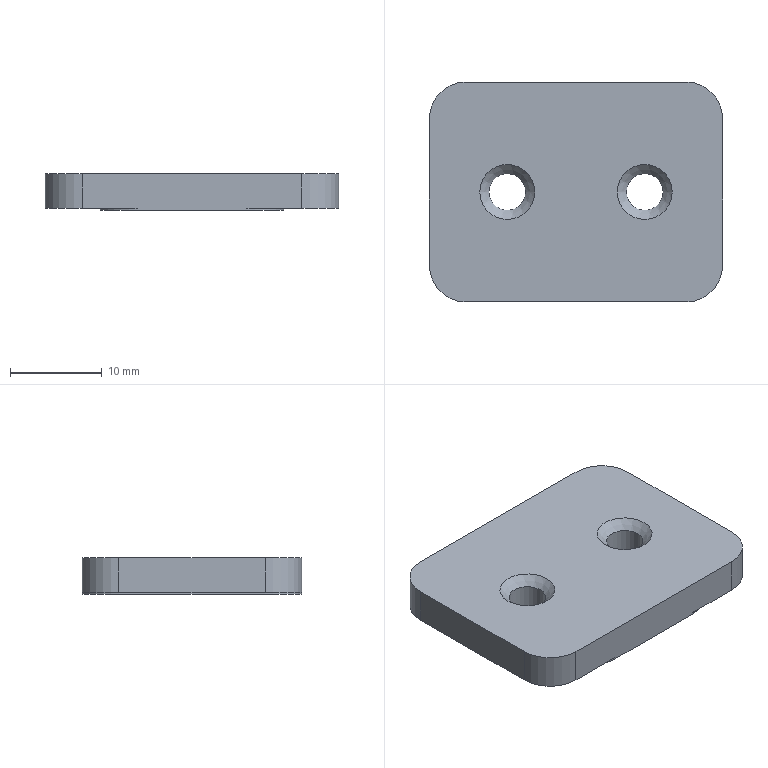Part | NX | features BREP 1, DATUM_CSYS 1 | 1 solid | 22 faces | box 32 x 24 x 4 mm | volume 2844 mm3 | plane 10 | cylinder 10 | cone 2 | commonest cylinder face diameters 8 x8 4 x2
STEP:
#1=CARTESIAN_POINT('',(16.,-8.,0.));
#2=VERTEX_POINT('',#1);
#3=CARTESIAN_POINT('',(16.,8.,0.));
#4=VERTEX_POINT('',#3);
#5=CARTESIAN_POINT('',(16.,-8.,0.));
#6=DIRECTION('',(0.,1.,0.));
#7=VECTOR('',#6,1000.);
#8=LINE('',#5,#7);
#9=EDGE_CURVE('',#2,#4,#8,.T.);
#10=ORIENTED_EDGE('',*,*,#9,.T.);
#11=CARTESIAN_POINT('',(12.,12.,0.));
#12=VERTEX_POINT('',#11);
#13=CARTESIAN_POINT('',(12.,8.,0.));
#14=DIRECTION('',(0.,0.,1.));
#15=DIRECTION('',(1.,0.,0.));
#16=AXIS2_PLACEMENT_3D('',#13,#14,#15);
#17=CIRCLE('',#16,4.);
#18=EDGE_CURVE('',#4,#12,#17,.T.);
#19=ORIENTED_EDGE('',*,*,#18,.T.);
#20=CARTESIAN_POINT('',(-12.,12.,0.));
#21=VERTEX_POINT('',#20);
#22=CARTESIAN_POINT('',(12.,12.,0.));
#23=DIRECTION('',(-1.,0.,0.));
#24=VECTOR('',#23,1000.);
#25=LINE('',#22,#24);
#26=EDGE_CURVE('',#12,#21,#25,.T.);
#27=ORIENTED_EDGE('',*,*,#26,.T.);
#28=CARTESIAN_POINT('',(-16.,8.,0.));
#29=VERTEX_POINT('',#28);
#30=CARTESIAN_POINT('',(-12.,8.,0.));
#31=DIRECTION('',(0.,0.,1.));
#32=DIRECTION('',(0.,1.,0.));
#33=AXIS2_PLACEMENT_3D('',#30,#31,#32);
#34=CIRCLE('',#33,4.);
#35=EDGE_CURVE('',#21,#29,#34,.T.);
#36=ORIENTED_EDGE('',*,*,#35,.T.);
#37=CARTESIAN_POINT('',(-16.,-8.,0.));
#38=VERTEX_POINT('',#37);
#39=CARTESIAN_POINT('',(-16.,8.,0.));
#40=DIRECTION('',(0.,-1.,0.));
#41=VECTOR('',#40,1000.);
#42=LINE('',#39,#41);
#43=EDGE_CURVE('',#29,#38,#42,.T.);
#44=ORIENTED_EDGE('',*,*,#43,.T.);
#45=CARTESIAN_POINT('',(-12.,-12.,0.));
#46=VERTEX_POINT('',#45);
#47=CARTESIAN_POINT('',(-12.,-8.,0.));
#48=DIRECTION('',(0.,0.,1.));
#49=DIRECTION('',(-1.,0.,0.));
#50=AXIS2_PLACEMENT_3D('',#47,#48,#49);
#51=CIRCLE('',#50,4.);
#52=EDGE_CURVE('',#38,#46,#51,.T.);
#53=ORIENTED_EDGE('',*,*,#52,.T.);
#54=CARTESIAN_POINT('',(12.,-12.,0.));
#55=VERTEX_POINT('',#54);
#56=CARTESIAN_POINT('',(-12.,-12.,0.));
#57=DIRECTION('',(1.,0.,0.));
#58=VECTOR('',#57,1000.);
#59=LINE('',#56,#58);
#60=EDGE_CURVE('',#46,#55,#59,.T.);
#61=ORIENTED_EDGE('',*,*,#60,.T.);
#62=CARTESIAN_POINT('',(12.,-8.,0.));
#63=DIRECTION('',(0.,0.,1.));
#64=DIRECTION('',(0.,-1.,0.));
#65=AXIS2_PLACEMENT_3D('',#62,#63,#64);
#66=CIRCLE('',#65,4.);
#67=EDGE_CURVE('',#55,#2,#66,.T.);
#68=ORIENTED_EDGE('',*,*,#67,.T.);
#69=EDGE_LOOP('',(#10,#19,#27,#36,#44,#53,#61,#68));
#70=FACE_BOUND('',#69,.T.);
#71=CARTESIAN_POINT('',(10.5,0.,0.));
#72=VERTEX_POINT('',#71);
#73=CARTESIAN_POINT('',(7.5,0.,0.));
#74=DIRECTION('',(0.,0.,-1.));
#75=DIRECTION('',(1.,0.,0.));
#76=AXIS2_PLACEMENT_3D('',#73,#74,#75);
#77=CIRCLE('',#76,3.);
#78=EDGE_CURVE('',#72,#72,#77,.T.);
#79=ORIENTED_EDGE('',*,*,#78,.T.);
#80=EDGE_LOOP('',(#79));
#81=FACE_BOUND('',#80,.T.);
#82=CARTESIAN_POINT('',(-4.5,0.,0.));
#83=VERTEX_POINT('',#82);
#84=CARTESIAN_POINT('',(-7.5,0.,0.));
#85=DIRECTION('',(0.,0.,-1.));
#86=DIRECTION('',(1.,0.,0.));
#87=AXIS2_PLACEMENT_3D('',#84,#85,#86);
#88=CIRCLE('',#87,3.);
#89=EDGE_CURVE('',#83,#83,#88,.T.);
#90=ORIENTED_EDGE('',*,*,#89,.T.);
#91=EDGE_LOOP('',(#90));
#92=FACE_BOUND('',#91,.T.);
#93=CARTESIAN_POINT('',(0.,4.,0.));
#94=DIRECTION('',(0.,0.,1.));
#95=DIRECTION('',(-1.,0.,0.));
#96=AXIS2_PLACEMENT_3D('',#93,#94,#95);
#97=PLANE('',#96);
#98=ADVANCED_FACE('',(#70,#81,#92),#97,.T.);
#99=CARTESIAN_POINT('',(16.,-8.,-3.8));
#100=VERTEX_POINT('',#99);
#101=CARTESIAN_POINT('',(16.,-8.,0.));
#102=DIRECTION('',(0.,0.,-1.));
#103=VECTOR('',#102,1000.);
#104=LINE('',#101,#103);
#105=EDGE_CURVE('',#2,#100,#104,.T.);
#106=ORIENTED_EDGE('',*,*,#105,.T.);
#107=CARTESIAN_POINT('',(16.,8.,-3.8));
#108=VERTEX_POINT('',#107);
#109=CARTESIAN_POINT('',(16.,-8.,-3.8));
#110=DIRECTION('',(0.,1.,0.));
#111=VECTOR('',#110,1000.);
#112=LINE('',#109,#111);
#113=EDGE_CURVE('',#100,#108,#112,.T.);
#114=ORIENTED_EDGE('',*,*,#113,.T.);
#115=CARTESIAN_POINT('',(16.,8.,0.));
#116=DIRECTION('',(0.,0.,-1.));
#117=VECTOR('',#116,1000.);
#118=LINE('',#115,#117);
#119=EDGE_CURVE('',#4,#108,#118,.T.);
#120=ORIENTED_EDGE('',*,*,#119,.F.);
#121=ORIENTED_EDGE('',*,*,#9,.F.);
#122=EDGE_LOOP('',(#106,#114,#120,#121));
#123=FACE_BOUND('',#122,.T.);
#124=CARTESIAN_POINT('',(16.,0.,-1.9));
#125=DIRECTION('',(-1.,0.,0.));
#126=DIRECTION('',(0.,-1.,0.));
#127=AXIS2_PLACEMENT_3D('',#124,#125,#126);
#128=PLANE('',#127);
#129=ADVANCED_FACE('',(#123),#128,.F.);
#130=ORIENTED_EDGE('',*,*,#119,.T.);
#131=CARTESIAN_POINT('',(12.,12.,-3.8));
#132=VERTEX_POINT('',#131);
#133=CARTESIAN_POINT('',(12.,8.,-3.8));
#134=DIRECTION('',(0.,0.,1.));
#135=DIRECTION('',(1.,0.,0.));
#136=AXIS2_PLACEMENT_3D('',#133,#134,#135);
#137=CIRCLE('',#136,4.);
#138=EDGE_CURVE('',#108,#132,#137,.T.);
#139=ORIENTED_EDGE('',*,*,#138,.T.);
#140=CARTESIAN_POINT('',(12.,12.,0.));
#141=DIRECTION('',(0.,0.,-1.));
#142=VECTOR('',#141,1000.);
#143=LINE('',#140,#142);
#144=EDGE_CURVE('',#12,#132,#143,.T.);
#145=ORIENTED_EDGE('',*,*,#144,.F.);
#146=ORIENTED_EDGE('',*,*,#18,.F.);
#147=EDGE_LOOP('',(#130,#139,#145,#146));
#148=FACE_BOUND('',#147,.T.);
#149=CARTESIAN_POINT('',(12.,8.,0.));
#150=DIRECTION('',(0.,0.,-1.));
#151=DIRECTION('',(-1.,0.,0.));
#152=AXIS2_PLACEMENT_3D('',#149,#150,#151);
#153=CYLINDRICAL_SURFACE('',#152,4.);
#154=ADVANCED_FACE('',(#148),#153,.T.);
#155=ORIENTED_EDGE('',*,*,#144,.T.);
#156=CARTESIAN_POINT('',(6.,12.,-3.8));
#157=VERTEX_POINT('',#156);
#158=CARTESIAN_POINT('',(12.,12.,-3.8));
#159=DIRECTION('',(-1.,0.,0.));
#160=VECTOR('',#159,1000.);
#161=LINE('',#158,#160);
#162=EDGE_CURVE('',#132,#157,#161,.T.);
#163=ORIENTED_EDGE('',*,*,#162,.T.);
#164=CARTESIAN_POINT('',(6.,12.,-4.));
#165=VERTEX_POINT('',#164);
#166=CARTESIAN_POINT('',(6.,12.,-3.8));
#167=DIRECTION('',(0.,0.,-1.));
#168=VECTOR('',#167,1000.);
#169=LINE('',#166,#168);
#170=EDGE_CURVE('',#157,#165,#169,.T.);
#171=ORIENTED_EDGE('',*,*,#170,.T.);
#172=CARTESIAN_POINT('',(-6.,12.,-4.));
#173=VERTEX_POINT('',#172);
#174=CARTESIAN_POINT('',(-6.,12.,-4.));
#175=DIRECTION('',(1.,0.,0.));
#176=VECTOR('',#175,1000.);
#177=LINE('',#174,#176);
#178=EDGE_CURVE('',#173,#165,#177,.T.);
#179=ORIENTED_EDGE('',*,*,#178,.F.);
#180=CARTESIAN_POINT('',(-6.,12.,-3.8));
#181=VERTEX_POINT('',#180);
#182=CARTESIAN_POINT('',(-6.,12.,-3.8));
#183=DIRECTION('',(0.,0.,-1.));
#184=VECTOR('',#183,1000.);
#185=LINE('',#182,#184);
#186=EDGE_CURVE('',#181,#173,#185,.T.);
#187=ORIENTED_EDGE('',*,*,#186,.F.);
#188=CARTESIAN_POINT('',(-12.,12.,-3.8));
#189=VERTEX_POINT('',#188);
#190=CARTESIAN_POINT('',(-6.,12.,-3.8));
#191=DIRECTION('',(-1.,0.,0.));
#192=VECTOR('',#191,1000.);
#193=LINE('',#190,#192);
#194=EDGE_CURVE('',#181,#189,#193,.T.);
#195=ORIENTED_EDGE('',*,*,#194,.T.);
#196=CARTESIAN_POINT('',(-12.,12.,0.));
#197=DIRECTION('',(0.,0.,-1.));
#198=VECTOR('',#197,1000.);
#199=LINE('',#196,#198);
#200=EDGE_CURVE('',#21,#189,#199,.T.);
#201=ORIENTED_EDGE('',*,*,#200,.F.);
#202=ORIENTED_EDGE('',*,*,#26,.F.);
#203=EDGE_LOOP('',(#155,#163,#171,#179,#187,#195,#201,#202));
#204=FACE_BOUND('',#203,.T.);
#205=CARTESIAN_POINT('',(0.,12.,-2.));
#206=DIRECTION('',(0.,-1.,0.));
#207=DIRECTION('',(1.,0.,0.));
#208=AXIS2_PLACEMENT_3D('',#205,#206,#207);
#209=PLANE('',#208);
#210=ADVANCED_FACE('',(#204),#209,.F.);
#211=ORIENTED_EDGE('',*,*,#200,.T.);
#212=CARTESIAN_POINT('',(-16.,8.,-3.8));
#213=VERTEX_POINT('',#212);
#214=CARTESIAN_POINT('',(-12.,8.,-3.8));
#215=DIRECTION('',(0.,0.,1.));
#216=DIRECTION('',(0.,1.,0.));
#217=AXIS2_PLACEMENT_3D('',#214,#215,#216);
#218=CIRCLE('',#217,4.);
#219=EDGE_CURVE('',#189,#213,#218,.T.);
#220=ORIENTED_EDGE('',*,*,#219,.T.);
#221=CARTESIAN_POINT('',(-16.,8.,0.));
#222=DIRECTION('',(0.,0.,-1.));
#223=VECTOR('',#222,1000.);
#224=LINE('',#221,#223);
#225=EDGE_CURVE('',#29,#213,#224,.T.);
#226=ORIENTED_EDGE('',*,*,#225,.F.);
#227=ORIENTED_EDGE('',*,*,#35,.F.);
#228=EDGE_LOOP('',(#211,#220,#226,#227));
#229=FACE_BOUND('',#228,.T.);
#230=CARTESIAN_POINT('',(-12.,8.,0.));
#231=DIRECTION('',(0.,0.,-1.));
#232=DIRECTION('',(0.,-1.,0.));
#233=AXIS2_PLACEMENT_3D('',#230,#231,#232);
#234=CYLINDRICAL_SURFACE('',#233,4.);
#235=ADVANCED_FACE('',(#229),#234,.T.);
#236=ORIENTED_EDGE('',*,*,#225,.T.);
#237=CARTESIAN_POINT('',(-16.,-8.,-3.8));
#238=VERTEX_POINT('',#237);
#239=CARTESIAN_POINT('',(-16.,8.,-3.8));
#240=DIRECTION('',(0.,-1.,0.));
#241=VECTOR('',#240,1000.);
#242=LINE('',#239,#241);
#243=EDGE_CURVE('',#213,#238,#242,.T.);
#244=ORIENTED_EDGE('',*,*,#243,.T.);
#245=CARTESIAN_POINT('',(-16.,-8.,0.));
#246=DIRECTION('',(0.,0.,-1.));
#247=VECTOR('',#246,1000.);
#248=LINE('',#245,#247);
#249=EDGE_CURVE('',#38,#238,#248,.T.);
#250=ORIENTED_EDGE('',*,*,#249,.F.);
#251=ORIENTED_EDGE('',*,*,#43,.F.);
#252=EDGE_LOOP('',(#236,#244,#250,#251));
#253=FACE_BOUND('',#252,.T.);
#254=CARTESIAN_POINT('',(-16.,0.,-1.9));
#255=DIRECTION('',(1.,0.,0.));
#256=DIRECTION('',(0.,1.,0.));
#257=AXIS2_PLACEMENT_3D('',#254,#255,#256);
#258=PLANE('',#257);
#259=ADVANCED_FACE('',(#253),#258,.F.);
#260=ORIENTED_EDGE('',*,*,#249,.T.);
#261=CARTESIAN_POINT('',(-12.,-12.,-3.8));
#262=VERTEX_POINT('',#261);
#263=CARTESIAN_POINT('',(-12.,-8.,-3.8));
#264=DIRECTION('',(0.,0.,1.));
#265=DIRECTION('',(-1.,0.,0.));
#266=AXIS2_PLACEMENT_3D('',#263,#264,#265);
#267=CIRCLE('',#266,4.);
#268=EDGE_CURVE('',#238,#262,#267,.T.);
#269=ORIENTED_EDGE('',*,*,#268,.T.);
#270=CARTESIAN_POINT('',(-12.,-12.,0.));
#271=DIRECTION('',(0.,0.,-1.));
#272=VECTOR('',#271,1000.);
#273=LINE('',#270,#272);
#274=EDGE_CURVE('',#46,#262,#273,.T.);
#275=ORIENTED_EDGE('',*,*,#274,.F.);
#276=ORIENTED_EDGE('',*,*,#52,.F.);
#277=EDGE_LOOP('',(#260,#269,#275,#276));
#278=FACE_BOUND('',#277,.T.);
#279=CARTESIAN_POINT('',(-12.,-8.,0.));
#280=DIRECTION('',(0.,0.,-1.));
#281=DIRECTION('',(1.,0.,0.));
#282=AXIS2_PLACEMENT_3D('',#279,#280,#281);
#283=CYLINDRICAL_SURFACE('',#282,4.);
#284=ADVANCED_FACE('',(#278),#283,.T.);
#285=ORIENTED_EDGE('',*,*,#274,.T.);
#286=CARTESIAN_POINT('',(-6.,-12.,-3.8));
#287=VERTEX_POINT('',#286);
#288=CARTESIAN_POINT('',(-12.,-12.,-3.8));
#289=DIRECTION('',(1.,0.,0.));
#290=VECTOR('',#289,1000.);
#291=LINE('',#288,#290);
#292=EDGE_CURVE('',#262,#287,#291,.T.);
#293=ORIENTED_EDGE('',*,*,#292,.T.);
#294=CARTESIAN_POINT('',(-6.,-12.,-4.));
#295=VERTEX_POINT('',#294);
#296=CARTESIAN_POINT('',(-6.,-12.,-3.8));
#297=DIRECTION('',(0.,0.,-1.));
#298=VECTOR('',#297,1000.);
#299=LINE('',#296,#298);
#300=EDGE_CURVE('',#287,#295,#299,.T.);
#301=ORIENTED_EDGE('',*,*,#300,.T.);
#302=CARTESIAN_POINT('',(6.,-12.,-4.));
#303=VERTEX_POINT('',#302);
#304=CARTESIAN_POINT('',(6.,-12.,-4.));
#305=DIRECTION('',(-1.,0.,0.));
#306=VECTOR('',#305,1000.);
#307=LINE('',#304,#306);
#308=EDGE_CURVE('',#303,#295,#307,.T.);
#309=ORIENTED_EDGE('',*,*,#308,.F.);
#310=CARTESIAN_POINT('',(6.,-12.,-3.8));
#311=VERTEX_POINT('',#310);
#312=CARTESIAN_POINT('',(6.,-12.,-3.8));
#313=DIRECTION('',(0.,0.,-1.));
#314=VECTOR('',#313,1000.);
#315=LINE('',#312,#314);
#316=EDGE_CURVE('',#311,#303,#315,.T.);
#317=ORIENTED_EDGE('',*,*,#316,.F.);
#318=CARTESIAN_POINT('',(12.,-12.,-3.8));
#319=VERTEX_POINT('',#318);
#320=CARTESIAN_POINT('',(6.,-12.,-3.8));
#321=DIRECTION('',(1.,0.,0.));
#322=VECTOR('',#321,1000.);
#323=LINE('',#320,#322);
#324=EDGE_CURVE('',#311,#319,#323,.T.);
#325=ORIENTED_EDGE('',*,*,#324,.T.);
#326=CARTESIAN_POINT('',(12.,-12.,0.));
#327=DIRECTION('',(0.,0.,-1.));
#328=VECTOR('',#327,1000.);
#329=LINE('',#326,#328);
#330=EDGE_CURVE('',#55,#319,#329,.T.);
#331=ORIENTED_EDGE('',*,*,#330,.F.);
#332=ORIENTED_EDGE('',*,*,#60,.F.);
#333=EDGE_LOOP('',(#285,#293,#301,#309,#317,#325,#331,#332));
#334=FACE_BOUND('',#333,.T.);
#335=CARTESIAN_POINT('',(0.,-12.,-2.));
#336=DIRECTION('',(0.,1.,0.));
#337=DIRECTION('',(-1.,0.,0.));
#338=AXIS2_PLACEMENT_3D('',#335,#336,#337);
#339=PLANE('',#338);
#340=ADVANCED_FACE('',(#334),#339,.F.);
#341=ORIENTED_EDGE('',*,*,#330,.T.);
#342=CARTESIAN_POINT('',(12.,-8.,-3.8));
#343=DIRECTION('',(0.,0.,1.));
#344=DIRECTION('',(0.,-1.,0.));
#345=AXIS2_PLACEMENT_3D('',#342,#343,#344);
#346=CIRCLE('',#345,4.);
#347=EDGE_CURVE('',#319,#100,#346,.T.);
#348=ORIENTED_EDGE('',*,*,#347,.T.);
#349=ORIENTED_EDGE('',*,*,#105,.F.);
#350=ORIENTED_EDGE('',*,*,#67,.F.);
#351=EDGE_LOOP('',(#341,#348,#349,#350));
#352=FACE_BOUND('',#351,.T.);
#353=CARTESIAN_POINT('',(12.,-8.,0.));
#354=DIRECTION('',(0.,0.,-1.));
#355=DIRECTION('',(0.,1.,0.));
#356=AXIS2_PLACEMENT_3D('',#353,#354,#355);
#357=CYLINDRICAL_SURFACE('',#356,4.);
#358=ADVANCED_FACE('',(#352),#357,.T.);
#359=ORIENTED_EDGE('',*,*,#347,.F.);
#360=ORIENTED_EDGE('',*,*,#324,.F.);
#361=CARTESIAN_POINT('',(10.,-8.,-3.8));
#362=VERTEX_POINT('',#361);
#363=CARTESIAN_POINT('',(6.,-8.,-3.8));
#364=DIRECTION('',(0.,0.,-1.));
#365=DIRECTION('',(1.,0.,0.));
#366=AXIS2_PLACEMENT_3D('',#363,#364,#365);
#367=CIRCLE('',#366,4.);
#368=EDGE_CURVE('',#362,#311,#367,.T.);
#369=ORIENTED_EDGE('',*,*,#368,.F.);
#370=CARTESIAN_POINT('',(10.,8.,-3.8));
#371=VERTEX_POINT('',#370);
#372=CARTESIAN_POINT('',(10.,8.,-3.8));
#373=DIRECTION('',(0.,-1.,0.));
#374=VECTOR('',#373,1000.);
#375=LINE('',#372,#374);
#376=EDGE_CURVE('',#371,#362,#375,.T.);
#377=ORIENTED_EDGE('',*,*,#376,.F.);
#378=CARTESIAN_POINT('',(6.,8.,-3.8));
#379=DIRECTION('',(0.,0.,-1.));
#380=DIRECTION('',(0.,1.,0.));
#381=AXIS2_PLACEMENT_3D('',#378,#379,#380);
#382=CIRCLE('',#381,4.);
#383=EDGE_CURVE('',#157,#371,#382,.T.);
#384=ORIENTED_EDGE('',*,*,#383,.F.);
#385=ORIENTED_EDGE('',*,*,#162,.F.);
#386=ORIENTED_EDGE('',*,*,#138,.F.);
#387=ORIENTED_EDGE('',*,*,#113,.F.);
#388=EDGE_LOOP('',(#359,#360,#369,#377,#384,#385,#386,#387));
#389=FACE_BOUND('',#388,.T.);
#390=CARTESIAN_POINT('',(0.,0.,-3.8));
#391=DIRECTION('',(0.,0.,1.));
#392=DIRECTION('',(-1.,0.,0.));
#393=AXIS2_PLACEMENT_3D('',#390,#391,#392);
#394=PLANE('',#393);
#395=ADVANCED_FACE('',(#389),#394,.F.);
#396=ORIENTED_EDGE('',*,*,#194,.F.);
#397=CARTESIAN_POINT('',(-10.,8.,-3.8));
#398=VERTEX_POINT('',#397);
#399=CARTESIAN_POINT('',(-6.,8.,-3.8));
#400=DIRECTION('',(0.,0.,-1.));
#401=DIRECTION('',(-1.,0.,0.));
#402=AXIS2_PLACEMENT_3D('',#399,#400,#401);
#403=CIRCLE('',#402,4.);
#404=EDGE_CURVE('',#398,#181,#403,.T.);
#405=ORIENTED_EDGE('',*,*,#404,.F.);
#406=CARTESIAN_POINT('',(-10.,-8.,-3.8));
#407=VERTEX_POINT('',#406);
#408=CARTESIAN_POINT('',(-10.,-8.,-3.8));
#409=DIRECTION('',(0.,1.,0.));
#410=VECTOR('',#409,1000.);
#411=LINE('',#408,#410);
#412=EDGE_CURVE('',#407,#398,#411,.T.);
#413=ORIENTED_EDGE('',*,*,#412,.F.);
#414=CARTESIAN_POINT('',(-6.,-8.,-3.8));
#415=DIRECTION('',(0.,0.,-1.));
#416=DIRECTION('',(0.,-1.,0.));
#417=AXIS2_PLACEMENT_3D('',#414,#415,#416);
#418=CIRCLE('',#417,4.);
#419=EDGE_CURVE('',#287,#407,#418,.T.);
#420=ORIENTED_EDGE('',*,*,#419,.F.);
#421=ORIENTED_EDGE('',*,*,#292,.F.);
#422=ORIENTED_EDGE('',*,*,#268,.F.);
#423=ORIENTED_EDGE('',*,*,#243,.F.);
#424=ORIENTED_EDGE('',*,*,#219,.F.);
#425=EDGE_LOOP('',(#396,#405,#413,#420,#421,#422,#423,#424));
#426=FACE_BOUND('',#425,.T.);
#427=CARTESIAN_POINT('',(0.,0.,-3.8));
#428=DIRECTION('',(0.,0.,1.));
#429=DIRECTION('',(-1.,0.,0.));
#430=AXIS2_PLACEMENT_3D('',#427,#428,#429);
#431=PLANE('',#430);
#432=ADVANCED_FACE('',(#426),#431,.F.);
#433=ORIENTED_EDGE('',*,*,#383,.T.);
#434=CARTESIAN_POINT('',(10.,8.,-4.));
#435=VERTEX_POINT('',#434);
#436=CARTESIAN_POINT('',(10.,8.,-3.8));
#437=DIRECTION('',(0.,0.,-1.));
#438=VECTOR('',#437,1000.);
#439=LINE('',#436,#438);
#440=EDGE_CURVE('',#371,#435,#439,.T.);
#441=ORIENTED_EDGE('',*,*,#440,.T.);
#442=CARTESIAN_POINT('',(6.,8.,-4.));
#443=DIRECTION('',(0.,0.,-1.));
#444=DIRECTION('',(0.,1.,0.));
#445=AXIS2_PLACEMENT_3D('',#442,#443,#444);
#446=CIRCLE('',#445,4.);
#447=EDGE_CURVE('',#165,#435,#446,.T.);
#448=ORIENTED_EDGE('',*,*,#447,.F.);
#449=ORIENTED_EDGE('',*,*,#170,.F.);
#450=EDGE_LOOP('',(#433,#441,#448,#449));
#451=FACE_BOUND('',#450,.T.);
#452=CARTESIAN_POINT('',(6.,8.,-3.8));
#453=DIRECTION('',(0.,0.,-1.));
#454=DIRECTION('',(0.,-1.,0.));
#455=AXIS2_PLACEMENT_3D('',#452,#453,#454);
#456=CYLINDRICAL_SURFACE('',#455,4.);
#457=ADVANCED_FACE('',(#451),#456,.T.);
#458=ORIENTED_EDGE('',*,*,#376,.T.);
#459=CARTESIAN_POINT('',(10.,-8.,-4.));
#460=VERTEX_POINT('',#459);
#461=CARTESIAN_POINT('',(10.,-8.,-3.8));
#462=DIRECTION('',(0.,0.,-1.));
#463=VECTOR('',#462,1000.);
#464=LINE('',#461,#463);
#465=EDGE_CURVE('',#362,#460,#464,.T.);
#466=ORIENTED_EDGE('',*,*,#465,.T.);
#467=CARTESIAN_POINT('',(10.,8.,-4.));
#468=DIRECTION('',(0.,-1.,0.));
#469=VECTOR('',#468,1000.);
#470=LINE('',#467,#469);
#471=EDGE_CURVE('',#435,#460,#470,.T.);
#472=ORIENTED_EDGE('',*,*,#471,.F.);
#473=ORIENTED_EDGE('',*,*,#440,.F.);
#474=EDGE_LOOP('',(#458,#466,#472,#473));
#475=FACE_BOUND('',#474,.T.);
#476=CARTESIAN_POINT('',(10.,0.,-3.9));
#477=DIRECTION('',(1.,0.,0.));
#478=DIRECTION('',(0.,1.,0.));
#479=AXIS2_PLACEMENT_3D('',#476,#477,#478);
#480=PLANE('',#479);
#481=ADVANCED_FACE('',(#475),#480,.T.);
#482=ORIENTED_EDGE('',*,*,#368,.T.);
#483=ORIENTED_EDGE('',*,*,#316,.T.);
#484=CARTESIAN_POINT('',(6.,-8.,-4.));
#485=DIRECTION('',(0.,0.,-1.));
#486=DIRECTION('',(1.,0.,0.));
#487=AXIS2_PLACEMENT_3D('',#484,#485,#486);
#488=CIRCLE('',#487,4.);
#489=EDGE_CURVE('',#460,#303,#488,.T.);
#490=ORIENTED_EDGE('',*,*,#489,.F.);
#491=ORIENTED_EDGE('',*,*,#465,.F.);
#492=EDGE_LOOP('',(#482,#483,#490,#491));
#493=FACE_BOUND('',#492,.T.);
#494=CARTESIAN_POINT('',(6.,-8.,-3.8));
#495=DIRECTION('',(0.,0.,-1.));
#496=DIRECTION('',(-1.,0.,0.));
#497=AXIS2_PLACEMENT_3D('',#494,#495,#496);
#498=CYLINDRICAL_SURFACE('',#497,4.);
#499=ADVANCED_FACE('',(#493),#498,.T.);
#500=ORIENTED_EDGE('',*,*,#419,.T.);
#501=CARTESIAN_POINT('',(-10.,-8.,-4.));
#502=VERTEX_POINT('',#501);
#503=CARTESIAN_POINT('',(-10.,-8.,-3.8));
#504=DIRECTION('',(0.,0.,-1.));
#505=VECTOR('',#504,1000.);
#506=LINE('',#503,#505);
#507=EDGE_CURVE('',#407,#502,#506,.T.);
#508=ORIENTED_EDGE('',*,*,#507,.T.);
#509=CARTESIAN_POINT('',(-6.,-8.,-4.));
#510=DIRECTION('',(0.,0.,-1.));
#511=DIRECTION('',(0.,-1.,0.));
#512=AXIS2_PLACEMENT_3D('',#509,#510,#511);
#513=CIRCLE('',#512,4.);
#514=EDGE_CURVE('',#295,#502,#513,.T.);
#515=ORIENTED_EDGE('',*,*,#514,.F.);
#516=ORIENTED_EDGE('',*,*,#300,.F.);
#517=EDGE_LOOP('',(#500,#508,#515,#516));
#518=FACE_BOUND('',#517,.T.);
#519=CARTESIAN_POINT('',(-6.,-8.,-3.8));
#520=DIRECTION('',(0.,0.,-1.));
#521=DIRECTION('',(0.,1.,0.));
#522=AXIS2_PLACEMENT_3D('',#519,#520,#521);
#523=CYLINDRICAL_SURFACE('',#522,4.);
#524=ADVANCED_FACE('',(#518),#523,.T.);
#525=ORIENTED_EDGE('',*,*,#412,.T.);
#526=CARTESIAN_POINT('',(-10.,8.,-4.));
#527=VERTEX_POINT('',#526);
#528=CARTESIAN_POINT('',(-10.,8.,-3.8));
#529=DIRECTION('',(0.,0.,-1.));
#530=VECTOR('',#529,1000.);
#531=LINE('',#528,#530);
#532=EDGE_CURVE('',#398,#527,#531,.T.);
#533=ORIENTED_EDGE('',*,*,#532,.T.);
#534=CARTESIAN_POINT('',(-10.,-8.,-4.));
#535=DIRECTION('',(0.,1.,0.));
#536=VECTOR('',#535,1000.);
#537=LINE('',#534,#536);
#538=EDGE_CURVE('',#502,#527,#537,.T.);
#539=ORIENTED_EDGE('',*,*,#538,.F.);
#540=ORIENTED_EDGE('',*,*,#507,.F.);
#541=EDGE_LOOP('',(#525,#533,#539,#540));
#542=FACE_BOUND('',#541,.T.);
#543=CARTESIAN_POINT('',(-10.,0.,-3.9));
#544=DIRECTION('',(-1.,0.,0.));
#545=DIRECTION('',(0.,-1.,0.));
#546=AXIS2_PLACEMENT_3D('',#543,#544,#545);
#547=PLANE('',#546);
#548=ADVANCED_FACE('',(#542),#547,.T.);
#549=ORIENTED_EDGE('',*,*,#404,.T.);
#550=ORIENTED_EDGE('',*,*,#186,.T.);
#551=CARTESIAN_POINT('',(-6.,8.,-4.));
#552=DIRECTION('',(0.,0.,-1.));
#553=DIRECTION('',(-1.,0.,0.));
#554=AXIS2_PLACEMENT_3D('',#551,#552,#553);
#555=CIRCLE('',#554,4.);
#556=EDGE_CURVE('',#527,#173,#555,.T.);
#557=ORIENTED_EDGE('',*,*,#556,.F.);
#558=ORIENTED_EDGE('',*,*,#532,.F.);
#559=EDGE_LOOP('',(#549,#550,#557,#558));
#560=FACE_BOUND('',#559,.T.);
#561=CARTESIAN_POINT('',(-6.,8.,-3.8));
#562=DIRECTION('',(0.,0.,-1.));
#563=DIRECTION('',(1.,0.,0.));
#564=AXIS2_PLACEMENT_3D('',#561,#562,#563);
#565=CYLINDRICAL_SURFACE('',#564,4.);
#566=ADVANCED_FACE('',(#560),#565,.T.);
#567=ORIENTED_EDGE('',*,*,#556,.T.);
#568=ORIENTED_EDGE('',*,*,#178,.T.);
#569=ORIENTED_EDGE('',*,*,#447,.T.);
#570=ORIENTED_EDGE('',*,*,#471,.T.);
#571=ORIENTED_EDGE('',*,*,#489,.T.);
#572=ORIENTED_EDGE('',*,*,#308,.T.);
#573=ORIENTED_EDGE('',*,*,#514,.T.);
#574=ORIENTED_EDGE('',*,*,#538,.T.);
#575=EDGE_LOOP('',(#567,#568,#569,#570,#571,#572,#573,#574));
#576=FACE_BOUND('',#575,.T.);
#577=CARTESIAN_POINT('',(-5.5,0.,-4.));
#578=VERTEX_POINT('',#577);
#579=CARTESIAN_POINT('',(-7.5,0.,-4.));
#580=DIRECTION('',(0.,0.,-1.));
#581=DIRECTION('',(1.,0.,0.));
#582=AXIS2_PLACEMENT_3D('',#579,#580,#581);
#583=CIRCLE('',#582,2.);
#584=EDGE_CURVE('',#578,#578,#583,.T.);
#585=ORIENTED_EDGE('',*,*,#584,.F.);
#586=EDGE_LOOP('',(#585));
#587=FACE_BOUND('',#586,.T.);
#588=CARTESIAN_POINT('',(9.5,0.,-4.));
#589=VERTEX_POINT('',#588);
#590=CARTESIAN_POINT('',(7.5,0.,-4.));
#591=DIRECTION('',(0.,0.,-1.));
#592=DIRECTION('',(1.,0.,0.));
#593=AXIS2_PLACEMENT_3D('',#590,#591,#592);
#594=CIRCLE('',#593,2.);
#595=EDGE_CURVE('',#589,#589,#594,.T.);
#596=ORIENTED_EDGE('',*,*,#595,.F.);
#597=EDGE_LOOP('',(#596));
#598=FACE_BOUND('',#597,.T.);
#599=CARTESIAN_POINT('',(2.,0.,-4.));
#600=DIRECTION('',(0.,0.,-1.));
#601=DIRECTION('',(-1.,0.,0.));
#602=AXIS2_PLACEMENT_3D('',#599,#600,#601);
#603=PLANE('',#602);
#604=ADVANCED_FACE('',(#576,#587,#598),#603,.T.);
#605=CARTESIAN_POINT('',(9.5,0.,-1.));
#606=VERTEX_POINT('',#605);
#607=CARTESIAN_POINT('',(10.5,0.,0.));
#608=DIRECTION('',(-0.7071,0.,-0.7071));
#609=VECTOR('',#608,1000.);
#610=LINE('',#607,#609);
#611=EDGE_CURVE('',#72,#606,#610,.T.);
#612=ORIENTED_EDGE('',*,*,#611,.T.);
#613=CARTESIAN_POINT('',(7.5,0.,-1.));
#614=DIRECTION('',(0.,0.,-1.));
#615=DIRECTION('',(1.,0.,0.));
#616=AXIS2_PLACEMENT_3D('',#613,#614,#615);
#617=CIRCLE('',#616,2.);
#618=EDGE_CURVE('',#606,#606,#617,.T.);
#619=ORIENTED_EDGE('',*,*,#618,.T.);
#620=ORIENTED_EDGE('',*,*,#611,.F.);
#621=ORIENTED_EDGE('',*,*,#78,.F.);
#622=EDGE_LOOP('',(#612,#619,#620,#621));
#623=FACE_BOUND('',#622,.T.);
#624=CARTESIAN_POINT('',(7.5,0.,-1.));
#625=DIRECTION('',(0.,0.,1.));
#626=DIRECTION('',(-1.,0.,0.));
#627=AXIS2_PLACEMENT_3D('',#624,#625,#626);
#628=CONICAL_SURFACE('',#627,2.,0.7854);
#629=ADVANCED_FACE('',(#623),#628,.F.);
#630=CARTESIAN_POINT('',(-5.5,0.,-1.));
#631=VERTEX_POINT('',#630);
#632=CARTESIAN_POINT('',(-4.5,0.,0.));
#633=DIRECTION('',(-0.7071,0.,-0.7071));
#634=VECTOR('',#633,1000.);
#635=LINE('',#632,#634);
#636=EDGE_CURVE('',#83,#631,#635,.T.);
#637=ORIENTED_EDGE('',*,*,#636,.T.);
#638=CARTESIAN_POINT('',(-7.5,0.,-1.));
#639=DIRECTION('',(0.,0.,-1.));
#640=DIRECTION('',(1.,0.,0.));
#641=AXIS2_PLACEMENT_3D('',#638,#639,#640);
#642=CIRCLE('',#641,2.);
#643=EDGE_CURVE('',#631,#631,#642,.T.);
#644=ORIENTED_EDGE('',*,*,#643,.T.);
#645=ORIENTED_EDGE('',*,*,#636,.F.);
#646=ORIENTED_EDGE('',*,*,#89,.F.);
#647=EDGE_LOOP('',(#637,#644,#645,#646));
#648=FACE_BOUND('',#647,.T.);
#649=CARTESIAN_POINT('',(-7.5,0.,-1.));
#650=DIRECTION('',(0.,0.,1.));
#651=DIRECTION('',(-1.,0.,0.));
#652=AXIS2_PLACEMENT_3D('',#649,#650,#651);
#653=CONICAL_SURFACE('',#652,2.,0.7854);
#654=ADVANCED_FACE('',(#648),#653,.F.);
#655=CARTESIAN_POINT('',(9.5,0.,-1.));
#656=DIRECTION('',(0.,0.,-1.));
#657=VECTOR('',#656,1000.);
#658=LINE('',#655,#657);
#659=EDGE_CURVE('',#606,#589,#658,.T.);
#660=ORIENTED_EDGE('',*,*,#659,.T.);
#661=ORIENTED_EDGE('',*,*,#595,.T.);
#662=ORIENTED_EDGE('',*,*,#659,.F.);
#663=ORIENTED_EDGE('',*,*,#618,.F.);
#664=EDGE_LOOP('',(#660,#661,#662,#663));
#665=FACE_BOUND('',#664,.T.);
#666=CARTESIAN_POINT('',(7.5,0.,-1.));
#667=DIRECTION('',(0.,0.,-1.));
#668=DIRECTION('',(-1.,0.,0.));
#669=AXIS2_PLACEMENT_3D('',#666,#667,#668);
#670=CYLINDRICAL_SURFACE('',#669,2.);
#671=ADVANCED_FACE('',(#665),#670,.F.);
#672=CARTESIAN_POINT('',(-5.5,0.,-1.));
#673=DIRECTION('',(0.,0.,-1.));
#674=VECTOR('',#673,1000.);
#675=LINE('',#672,#674);
#676=EDGE_CURVE('',#631,#578,#675,.T.);
#677=ORIENTED_EDGE('',*,*,#676,.T.);
#678=ORIENTED_EDGE('',*,*,#584,.T.);
#679=ORIENTED_EDGE('',*,*,#676,.F.);
#680=ORIENTED_EDGE('',*,*,#643,.F.);
#681=EDGE_LOOP('',(#677,#678,#679,#680));
#682=FACE_BOUND('',#681,.T.);
#683=CARTESIAN_POINT('',(-7.5,0.,-1.));
#684=DIRECTION('',(0.,0.,-1.));
#685=DIRECTION('',(-1.,0.,0.));
#686=AXIS2_PLACEMENT_3D('',#683,#684,#685);
#687=CYLINDRICAL_SURFACE('',#686,2.);
#688=ADVANCED_FACE('',(#682),#687,.F.);
#689=CLOSED_SHELL('',(#98,#129,#154,#210,#235,#259,#284,#340,#358,#395,#432,#457,#481,#499,#524,#548,#566,#604,#629,#654,#671,#688));
#690=MANIFOLD_SOLID_BREP('',#689);
#691=(LENGTH_UNIT()NAMED_UNIT(*)SI_UNIT(.MILLI.,.METRE.));
#692=UNCERTAINTY_MEASURE_WITH_UNIT(LENGTH_MEASURE(0.00001),#691,'','');
#693=(NAMED_UNIT(*)PLANE_ANGLE_UNIT()SI_UNIT($,.RADIAN.));
#694=(NAMED_UNIT(*)SI_UNIT($,.STERADIAN.)SOLID_ANGLE_UNIT());
#695=(GEOMETRIC_REPRESENTATION_CONTEXT(3)GLOBAL_UNCERTAINTY_ASSIGNED_CONTEXT((#692))GLOBAL_UNIT_ASSIGNED_CONTEXT((#691,#693,#694))REPRESENTATION_CONTEXT('',''));
#696=ADVANCED_BREP_SHAPE_REPRESENTATION('',(#690),#695);